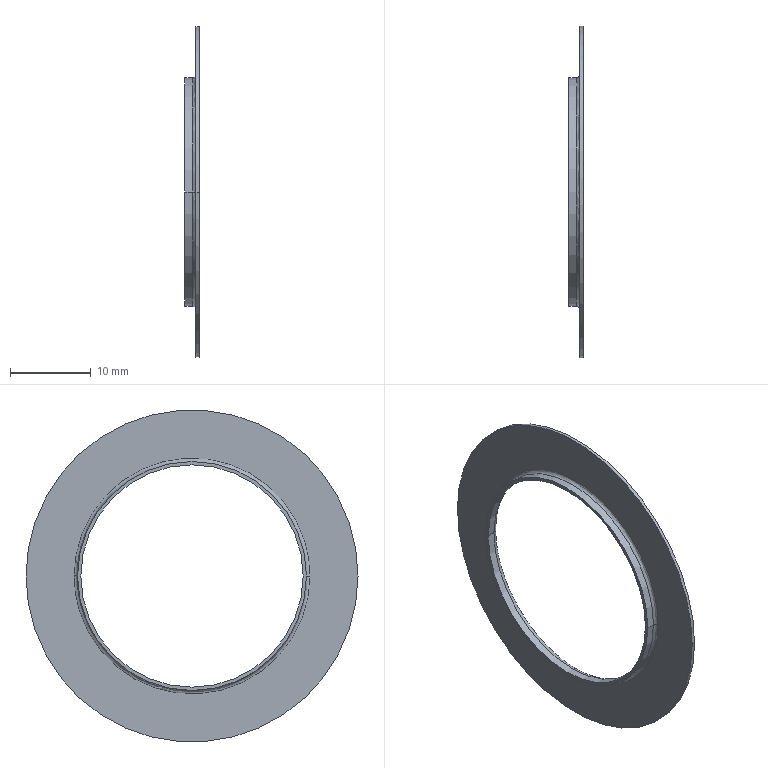Part | STEP file | Microwave Drying Flat Conveyor-inafag_ucfl204_62o9y6gnj3059x015y4y3bh4_11 | 1 solid | 13 faces | box 1.812 x 41.16 x 41.16 mm | volume 343.35 mm3 | cylinder 6 | spline 4 | plane 3 | commonest cylinder face diameters 27.56 x2 28.383 x2 41.16 x2